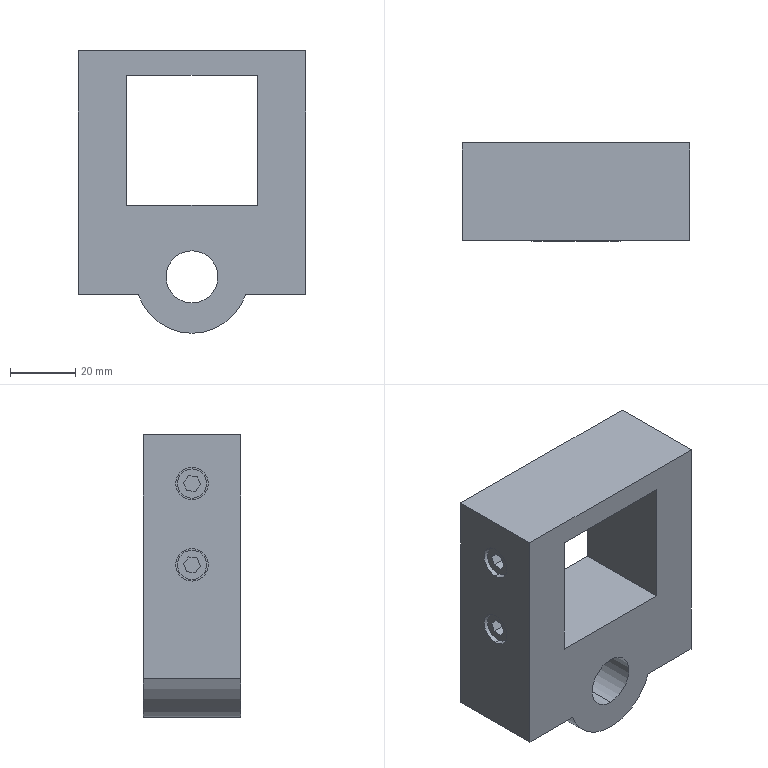Part | SolidWorks | features ICE 5, Extrusion 1, MirrorPattern 1 | 1 solid | 67 faces | box 70 x 30 x 86.838 mm | volume 111034 mm3 | plane 47 | cylinder 20 | commonest cylinder face diameters 9 x8 10 x8 16 x2 34.677 x2